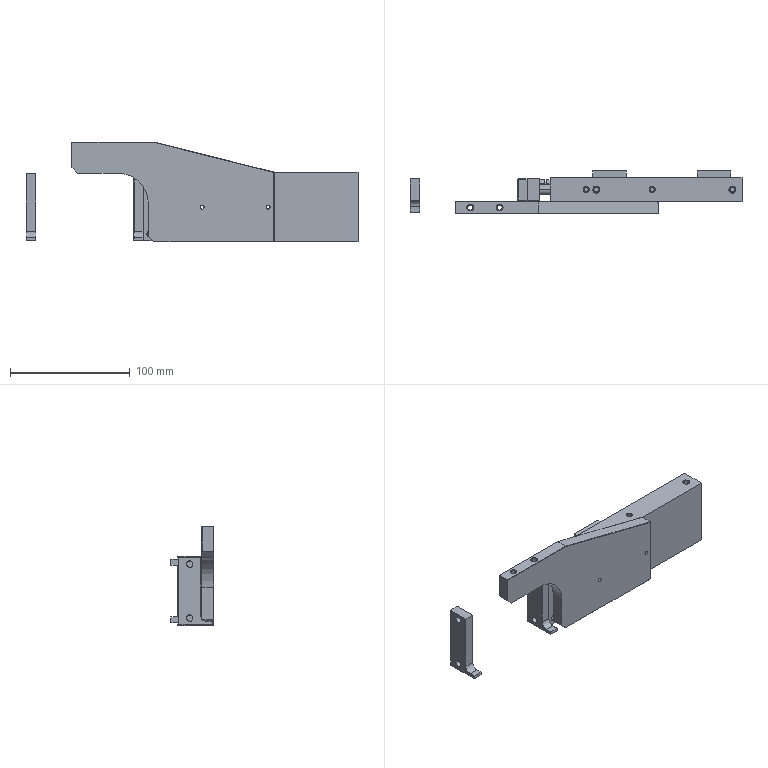Part | NX | 7 solids | 420 faces | box 277 x 36.196 x 83.25 mm | volume 290070 mm3 | plane 195 | cylinder 137 | cone 88 | commonest cylinder face diameters 4 x26 5 x18 3.4 x16 2.5 x12 8 x12 4.5 x8